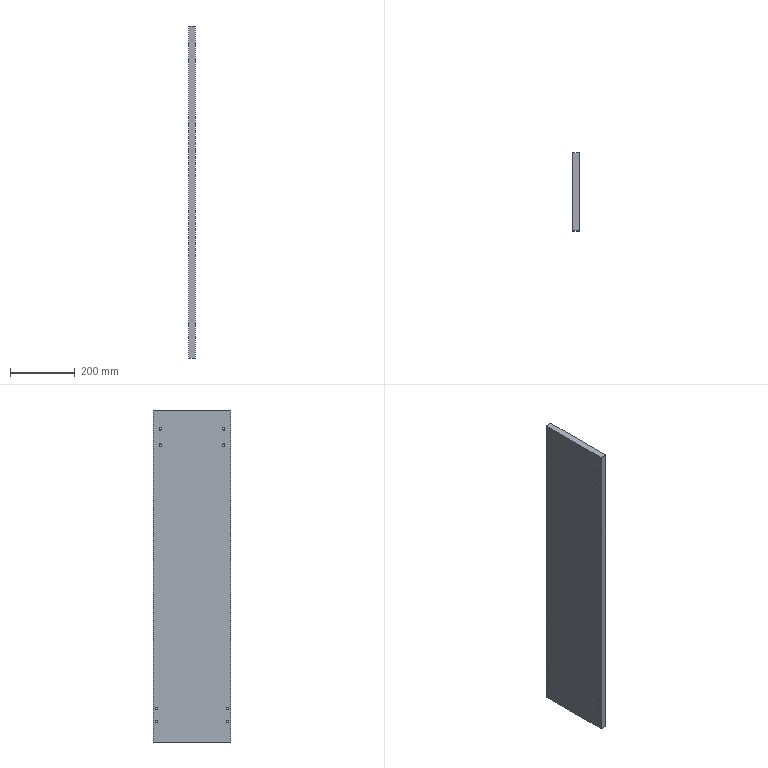Part | NX | features SIMPLE HOLE 8, SYMBOLIC_THREAD 8, LINKED_CURVE 4, DATUM_CSYS 3, SKETCH 2, EXTRUDE 1, HOLE PACKAGE 1, LINKED_FACE 1 | 1 solid | 30 faces | box 20 x 240 x 1027 mm | volume 4923724 mm3 | cone 16 | cylinder 8 | plane 6 | commonest cylinder face diameters 6.8 x8
STEP:
#1=CARTESIAN_POINT('',(85.,-120.,527.));
#2=VERTEX_POINT('',#1);
#3=CARTESIAN_POINT('',(85.,-120.,-500.));
#4=VERTEX_POINT('',#3);
#5=CARTESIAN_POINT('',(85.,-120.,527.));
#6=DIRECTION('',(0.,0.,-1.));
#7=VECTOR('',#6,1000.);
#8=LINE('',#5,#7);
#9=EDGE_CURVE('',#2,#4,#8,.T.);
#10=ORIENTED_EDGE('',*,*,#9,.T.);
#11=CARTESIAN_POINT('',(105.,-120.,-500.));
#12=VERTEX_POINT('',#11);
#13=CARTESIAN_POINT('',(105.,-120.,-500.));
#14=DIRECTION('',(-1.,0.,0.));
#15=VECTOR('',#14,1000.);
#16=LINE('',#13,#15);
#17=EDGE_CURVE('',#12,#4,#16,.T.);
#18=ORIENTED_EDGE('',*,*,#17,.F.);
#19=CARTESIAN_POINT('',(105.,-120.,527.));
#20=VERTEX_POINT('',#19);
#21=CARTESIAN_POINT('',(105.,-120.,527.));
#22=DIRECTION('',(0.,0.,-1.));
#23=VECTOR('',#22,1000.);
#24=LINE('',#21,#23);
#25=EDGE_CURVE('',#20,#12,#24,.T.);
#26=ORIENTED_EDGE('',*,*,#25,.F.);
#27=CARTESIAN_POINT('',(105.,-120.,527.));
#28=DIRECTION('',(-1.,0.,0.));
#29=VECTOR('',#28,1000.);
#30=LINE('',#27,#29);
#31=EDGE_CURVE('',#20,#2,#30,.T.);
#32=ORIENTED_EDGE('',*,*,#31,.T.);
#33=EDGE_LOOP('',(#10,#18,#26,#32));
#34=FACE_BOUND('',#33,.T.);
#35=CARTESIAN_POINT('',(105.,-120.,527.));
#36=DIRECTION('',(0.,1.,0.));
#37=DIRECTION('',(0.,0.,1.));
#38=AXIS2_PLACEMENT_3D('',#35,#36,#37);
#39=PLANE('',#38);
#40=ADVANCED_FACE('',(#34),#39,.F.);
#41=CARTESIAN_POINT('',(85.,120.,-500.));
#42=VERTEX_POINT('',#41);
#43=CARTESIAN_POINT('',(85.,-120.,-500.));
#44=DIRECTION('',(0.,1.,0.));
#45=VECTOR('',#44,1000.);
#46=LINE('',#43,#45);
#47=EDGE_CURVE('',#4,#42,#46,.T.);
#48=ORIENTED_EDGE('',*,*,#47,.T.);
#49=CARTESIAN_POINT('',(105.,120.,-500.));
#50=VERTEX_POINT('',#49);
#51=CARTESIAN_POINT('',(105.,120.,-500.));
#52=DIRECTION('',(-1.,0.,0.));
#53=VECTOR('',#52,1000.);
#54=LINE('',#51,#53);
#55=EDGE_CURVE('',#50,#42,#54,.T.);
#56=ORIENTED_EDGE('',*,*,#55,.F.);
#57=CARTESIAN_POINT('',(105.,-120.,-500.));
#58=DIRECTION('',(0.,1.,0.));
#59=VECTOR('',#58,1000.);
#60=LINE('',#57,#59);
#61=EDGE_CURVE('',#12,#50,#60,.T.);
#62=ORIENTED_EDGE('',*,*,#61,.F.);
#63=ORIENTED_EDGE('',*,*,#17,.T.);
#64=EDGE_LOOP('',(#48,#56,#62,#63));
#65=FACE_BOUND('',#64,.T.);
#66=CARTESIAN_POINT('',(105.,-120.,-500.));
#67=DIRECTION('',(0.,0.,1.));
#68=DIRECTION('',(1.,0.,0.));
#69=AXIS2_PLACEMENT_3D('',#66,#67,#68);
#70=PLANE('',#69);
#71=ADVANCED_FACE('',(#65),#70,.F.);
#72=CARTESIAN_POINT('',(85.,120.,527.));
#73=VERTEX_POINT('',#72);
#74=CARTESIAN_POINT('',(85.,120.,-500.));
#75=DIRECTION('',(0.,0.,1.));
#76=VECTOR('',#75,1000.);
#77=LINE('',#74,#76);
#78=EDGE_CURVE('',#42,#73,#77,.T.);
#79=ORIENTED_EDGE('',*,*,#78,.T.);
#80=CARTESIAN_POINT('',(105.,120.,527.));
#81=VERTEX_POINT('',#80);
#82=CARTESIAN_POINT('',(105.,120.,527.));
#83=DIRECTION('',(-1.,0.,0.));
#84=VECTOR('',#83,1000.);
#85=LINE('',#82,#84);
#86=EDGE_CURVE('',#81,#73,#85,.T.);
#87=ORIENTED_EDGE('',*,*,#86,.F.);
#88=CARTESIAN_POINT('',(105.,120.,-500.));
#89=DIRECTION('',(0.,0.,1.));
#90=VECTOR('',#89,1000.);
#91=LINE('',#88,#90);
#92=EDGE_CURVE('',#50,#81,#91,.T.);
#93=ORIENTED_EDGE('',*,*,#92,.F.);
#94=ORIENTED_EDGE('',*,*,#55,.T.);
#95=EDGE_LOOP('',(#79,#87,#93,#94));
#96=FACE_BOUND('',#95,.T.);
#97=CARTESIAN_POINT('',(105.,120.,-500.));
#98=DIRECTION('',(0.,-1.,0.));
#99=DIRECTION('',(0.,0.,-1.));
#100=AXIS2_PLACEMENT_3D('',#97,#98,#99);
#101=PLANE('',#100);
#102=ADVANCED_FACE('',(#96),#101,.F.);
#103=CARTESIAN_POINT('',(85.,120.,527.));
#104=DIRECTION('',(0.,-1.,0.));
#105=VECTOR('',#104,1000.);
#106=LINE('',#103,#105);
#107=EDGE_CURVE('',#73,#2,#106,.T.);
#108=ORIENTED_EDGE('',*,*,#107,.T.);
#109=ORIENTED_EDGE('',*,*,#31,.F.);
#110=CARTESIAN_POINT('',(105.,120.,527.));
#111=DIRECTION('',(0.,-1.,0.));
#112=VECTOR('',#111,1000.);
#113=LINE('',#110,#112);
#114=EDGE_CURVE('',#81,#20,#113,.T.);
#115=ORIENTED_EDGE('',*,*,#114,.F.);
#116=ORIENTED_EDGE('',*,*,#86,.T.);
#117=EDGE_LOOP('',(#108,#109,#115,#116));
#118=FACE_BOUND('',#117,.T.);
#119=CARTESIAN_POINT('',(105.,120.,527.));
#120=DIRECTION('',(0.,0.,-1.));
#121=DIRECTION('',(-1.,0.,0.));
#122=AXIS2_PLACEMENT_3D('',#119,#120,#121);
#123=PLANE('',#122);
#124=ADVANCED_FACE('',(#118),#123,.F.);
#125=CARTESIAN_POINT('',(105.,110.,-400.5));
#126=VERTEX_POINT('',#125);
#127=CARTESIAN_POINT('',(105.,110.,-396.5));
#128=DIRECTION('',(1.,0.,0.));
#129=DIRECTION('',(0.,0.,-1.));
#130=AXIS2_PLACEMENT_3D('',#127,#128,#129);
#131=CIRCLE('',#130,4.);
#132=EDGE_CURVE('',#126,#126,#131,.F.);
#133=ORIENTED_EDGE('',*,*,#132,.T.);
#134=EDGE_LOOP('',(#133));
#135=FACE_BOUND('',#134,.T.);
#136=CARTESIAN_POINT('',(105.,110.,-440.5));
#137=VERTEX_POINT('',#136);
#138=CARTESIAN_POINT('',(105.,110.,-436.5));
#139=DIRECTION('',(1.,0.,0.));
#140=DIRECTION('',(0.,0.,-1.));
#141=AXIS2_PLACEMENT_3D('',#138,#139,#140);
#142=CIRCLE('',#141,4.);
#143=EDGE_CURVE('',#137,#137,#142,.F.);
#144=ORIENTED_EDGE('',*,*,#143,.T.);
#145=EDGE_LOOP('',(#144));
#146=FACE_BOUND('',#145,.T.);
#147=CARTESIAN_POINT('',(105.,98.,464.5));
#148=VERTEX_POINT('',#147);
#149=CARTESIAN_POINT('',(105.,98.,468.5));
#150=DIRECTION('',(1.,0.,0.));
#151=DIRECTION('',(0.,0.,-1.));
#152=AXIS2_PLACEMENT_3D('',#149,#150,#151);
#153=CIRCLE('',#152,4.);
#154=EDGE_CURVE('',#148,#148,#153,.F.);
#155=ORIENTED_EDGE('',*,*,#154,.T.);
#156=EDGE_LOOP('',(#155));
#157=FACE_BOUND('',#156,.T.);
#158=CARTESIAN_POINT('',(105.,98.,414.5));
#159=VERTEX_POINT('',#158);
#160=CARTESIAN_POINT('',(105.,98.,418.5));
#161=DIRECTION('',(1.,0.,0.));
#162=DIRECTION('',(0.,0.,-1.));
#163=AXIS2_PLACEMENT_3D('',#160,#161,#162);
#164=CIRCLE('',#163,4.);
#165=EDGE_CURVE('',#159,#159,#164,.F.);
#166=ORIENTED_EDGE('',*,*,#165,.T.);
#167=EDGE_LOOP('',(#166));
#168=FACE_BOUND('',#167,.T.);
#169=CARTESIAN_POINT('',(105.,-98.,464.5));
#170=VERTEX_POINT('',#169);
#171=CARTESIAN_POINT('',(105.,-98.,468.5));
#172=DIRECTION('',(1.,0.,0.));
#173=DIRECTION('',(0.,0.,-1.));
#174=AXIS2_PLACEMENT_3D('',#171,#172,#173);
#175=CIRCLE('',#174,4.);
#176=EDGE_CURVE('',#170,#170,#175,.F.);
#177=ORIENTED_EDGE('',*,*,#176,.T.);
#178=EDGE_LOOP('',(#177));
#179=FACE_BOUND('',#178,.T.);
#180=CARTESIAN_POINT('',(105.,-98.,414.5));
#181=VERTEX_POINT('',#180);
#182=CARTESIAN_POINT('',(105.,-98.,418.5));
#183=DIRECTION('',(1.,0.,0.));
#184=DIRECTION('',(0.,0.,-1.));
#185=AXIS2_PLACEMENT_3D('',#182,#183,#184);
#186=CIRCLE('',#185,4.);
#187=EDGE_CURVE('',#181,#181,#186,.F.);
#188=ORIENTED_EDGE('',*,*,#187,.T.);
#189=EDGE_LOOP('',(#188));
#190=FACE_BOUND('',#189,.T.);
#191=CARTESIAN_POINT('',(105.,-110.,-400.5));
#192=VERTEX_POINT('',#191);
#193=CARTESIAN_POINT('',(105.,-110.,-396.5));
#194=DIRECTION('',(1.,0.,0.));
#195=DIRECTION('',(0.,0.,-1.));
#196=AXIS2_PLACEMENT_3D('',#193,#194,#195);
#197=CIRCLE('',#196,4.);
#198=EDGE_CURVE('',#192,#192,#197,.F.);
#199=ORIENTED_EDGE('',*,*,#198,.T.);
#200=EDGE_LOOP('',(#199));
#201=FACE_BOUND('',#200,.T.);
#202=CARTESIAN_POINT('',(105.,-110.,-440.5));
#203=VERTEX_POINT('',#202);
#204=CARTESIAN_POINT('',(105.,-110.,-436.5));
#205=DIRECTION('',(1.,0.,0.));
#206=DIRECTION('',(0.,0.,-1.));
#207=AXIS2_PLACEMENT_3D('',#204,#205,#206);
#208=CIRCLE('',#207,4.);
#209=EDGE_CURVE('',#203,#203,#208,.F.);
#210=ORIENTED_EDGE('',*,*,#209,.T.);
#211=EDGE_LOOP('',(#210));
#212=FACE_BOUND('',#211,.T.);
#213=ORIENTED_EDGE('',*,*,#25,.T.);
#214=ORIENTED_EDGE('',*,*,#61,.T.);
#215=ORIENTED_EDGE('',*,*,#92,.T.);
#216=ORIENTED_EDGE('',*,*,#114,.T.);
#217=EDGE_LOOP('',(#213,#214,#215,#216));
#218=FACE_BOUND('',#217,.T.);
#219=CARTESIAN_POINT('',(105.,0.,0.));
#220=DIRECTION('',(1.,0.,0.));
#221=DIRECTION('',(0.,0.,-1.));
#222=AXIS2_PLACEMENT_3D('',#219,#220,#221);
#223=PLANE('',#222);
#224=ADVANCED_FACE('',(#135,#146,#157,#168,#179,#190,#201,#212,#218),#223,.T.);
#225=CARTESIAN_POINT('',(85.,110.,-400.5));
#226=VERTEX_POINT('',#225);
#227=CARTESIAN_POINT('',(85.,110.,-396.5));
#228=DIRECTION('',(1.,0.,0.));
#229=DIRECTION('',(0.,0.,-1.));
#230=AXIS2_PLACEMENT_3D('',#227,#228,#229);
#231=CIRCLE('',#230,4.);
#232=EDGE_CURVE('',#226,#226,#231,.T.);
#233=ORIENTED_EDGE('',*,*,#232,.T.);
#234=EDGE_LOOP('',(#233));
#235=FACE_BOUND('',#234,.T.);
#236=CARTESIAN_POINT('',(85.,110.,-440.5));
#237=VERTEX_POINT('',#236);
#238=CARTESIAN_POINT('',(85.,110.,-436.5));
#239=DIRECTION('',(1.,0.,0.));
#240=DIRECTION('',(0.,0.,-1.));
#241=AXIS2_PLACEMENT_3D('',#238,#239,#240);
#242=CIRCLE('',#241,4.);
#243=EDGE_CURVE('',#237,#237,#242,.T.);
#244=ORIENTED_EDGE('',*,*,#243,.T.);
#245=EDGE_LOOP('',(#244));
#246=FACE_BOUND('',#245,.T.);
#247=CARTESIAN_POINT('',(85.,98.,464.5));
#248=VERTEX_POINT('',#247);
#249=CARTESIAN_POINT('',(85.,98.,468.5));
#250=DIRECTION('',(1.,0.,0.));
#251=DIRECTION('',(0.,0.,-1.));
#252=AXIS2_PLACEMENT_3D('',#249,#250,#251);
#253=CIRCLE('',#252,4.);
#254=EDGE_CURVE('',#248,#248,#253,.T.);
#255=ORIENTED_EDGE('',*,*,#254,.T.);
#256=EDGE_LOOP('',(#255));
#257=FACE_BOUND('',#256,.T.);
#258=CARTESIAN_POINT('',(85.,98.,414.5));
#259=VERTEX_POINT('',#258);
#260=CARTESIAN_POINT('',(85.,98.,418.5));
#261=DIRECTION('',(1.,0.,0.));
#262=DIRECTION('',(0.,0.,-1.));
#263=AXIS2_PLACEMENT_3D('',#260,#261,#262);
#264=CIRCLE('',#263,4.);
#265=EDGE_CURVE('',#259,#259,#264,.T.);
#266=ORIENTED_EDGE('',*,*,#265,.T.);
#267=EDGE_LOOP('',(#266));
#268=FACE_BOUND('',#267,.T.);
#269=CARTESIAN_POINT('',(85.,-98.,464.5));
#270=VERTEX_POINT('',#269);
#271=CARTESIAN_POINT('',(85.,-98.,468.5));
#272=DIRECTION('',(1.,0.,0.));
#273=DIRECTION('',(0.,0.,-1.));
#274=AXIS2_PLACEMENT_3D('',#271,#272,#273);
#275=CIRCLE('',#274,4.);
#276=EDGE_CURVE('',#270,#270,#275,.T.);
#277=ORIENTED_EDGE('',*,*,#276,.T.);
#278=EDGE_LOOP('',(#277));
#279=FACE_BOUND('',#278,.T.);
#280=CARTESIAN_POINT('',(85.,-98.,414.5));
#281=VERTEX_POINT('',#280);
#282=CARTESIAN_POINT('',(85.,-98.,418.5));
#283=DIRECTION('',(1.,0.,0.));
#284=DIRECTION('',(0.,0.,-1.));
#285=AXIS2_PLACEMENT_3D('',#282,#283,#284);
#286=CIRCLE('',#285,4.);
#287=EDGE_CURVE('',#281,#281,#286,.T.);
#288=ORIENTED_EDGE('',*,*,#287,.T.);
#289=EDGE_LOOP('',(#288));
#290=FACE_BOUND('',#289,.T.);
#291=CARTESIAN_POINT('',(85.,-110.,-400.5));
#292=VERTEX_POINT('',#291);
#293=CARTESIAN_POINT('',(85.,-110.,-396.5));
#294=DIRECTION('',(1.,0.,0.));
#295=DIRECTION('',(0.,0.,-1.));
#296=AXIS2_PLACEMENT_3D('',#293,#294,#295);
#297=CIRCLE('',#296,4.);
#298=EDGE_CURVE('',#292,#292,#297,.T.);
#299=ORIENTED_EDGE('',*,*,#298,.T.);
#300=EDGE_LOOP('',(#299));
#301=FACE_BOUND('',#300,.T.);
#302=CARTESIAN_POINT('',(85.,-110.,-440.5));
#303=VERTEX_POINT('',#302);
#304=CARTESIAN_POINT('',(85.,-110.,-436.5));
#305=DIRECTION('',(1.,0.,0.));
#306=DIRECTION('',(0.,0.,-1.));
#307=AXIS2_PLACEMENT_3D('',#304,#305,#306);
#308=CIRCLE('',#307,4.);
#309=EDGE_CURVE('',#303,#303,#308,.T.);
#310=ORIENTED_EDGE('',*,*,#309,.T.);
#311=EDGE_LOOP('',(#310));
#312=FACE_BOUND('',#311,.T.);
#313=ORIENTED_EDGE('',*,*,#9,.F.);
#314=ORIENTED_EDGE('',*,*,#107,.F.);
#315=ORIENTED_EDGE('',*,*,#78,.F.);
#316=ORIENTED_EDGE('',*,*,#47,.F.);
#317=EDGE_LOOP('',(#313,#314,#315,#316));
#318=FACE_BOUND('',#317,.T.);
#319=CARTESIAN_POINT('',(85.,0.,0.));
#320=DIRECTION('',(1.,0.,0.));
#321=DIRECTION('',(0.,0.,-1.));
#322=AXIS2_PLACEMENT_3D('',#319,#320,#321);
#323=PLANE('',#322);
#324=ADVANCED_FACE('',(#235,#246,#257,#268,#279,#290,#301,#312,#318),#323,.F.);
#325=CARTESIAN_POINT('',(104.4,-110.,-439.9));
#326=VERTEX_POINT('',#325);
#327=CARTESIAN_POINT('',(104.4,-110.,-436.5));
#328=DIRECTION('',(1.,0.,0.));
#329=DIRECTION('',(0.,0.,-1.));
#330=AXIS2_PLACEMENT_3D('',#327,#328,#329);
#331=CIRCLE('',#330,3.4);
#332=EDGE_CURVE('',#326,#326,#331,.T.);
#333=ORIENTED_EDGE('',*,*,#332,.T.);
#334=EDGE_LOOP('',(#333));
#335=FACE_BOUND('',#334,.T.);
#336=CARTESIAN_POINT('',(85.6,-110.,-439.9));
#337=VERTEX_POINT('',#336);
#338=CARTESIAN_POINT('',(85.6,-110.,-436.5));
#339=DIRECTION('',(1.,0.,0.));
#340=DIRECTION('',(0.,0.,-1.));
#341=AXIS2_PLACEMENT_3D('',#338,#339,#340);
#342=CIRCLE('',#341,3.4);
#343=EDGE_CURVE('',#337,#337,#342,.F.);
#344=ORIENTED_EDGE('',*,*,#343,.T.);
#345=EDGE_LOOP('',(#344));
#346=FACE_BOUND('',#345,.T.);
#347=CARTESIAN_POINT('',(85.,-110.,-436.5));
#348=DIRECTION('',(1.,0.,0.));
#349=DIRECTION('',(0.,0.,-1.));
#350=AXIS2_PLACEMENT_3D('',#347,#348,#349);
#351=CYLINDRICAL_SURFACE('',#350,3.4);
#352=ADVANCED_FACE('',(#335,#346),#351,.F.);
#353=ORIENTED_EDGE('',*,*,#343,.F.);
#354=EDGE_LOOP('',(#353));
#355=FACE_BOUND('',#354,.T.);
#356=ORIENTED_EDGE('',*,*,#309,.F.);
#357=EDGE_LOOP('',(#356));
#358=FACE_BOUND('',#357,.T.);
#359=CARTESIAN_POINT('',(85.,-110.,-436.5));
#360=DIRECTION('',(-1.,0.,0.));
#361=DIRECTION('',(0.,0.,1.));
#362=AXIS2_PLACEMENT_3D('',#359,#360,#361);
#363=CONICAL_SURFACE('',#362,4.,0.7854);
#364=ADVANCED_FACE('',(#355,#358),#363,.F.);
#365=ORIENTED_EDGE('',*,*,#209,.F.);
#366=EDGE_LOOP('',(#365));
#367=FACE_BOUND('',#366,.T.);
#368=ORIENTED_EDGE('',*,*,#332,.F.);
#369=EDGE_LOOP('',(#368));
#370=FACE_BOUND('',#369,.T.);
#371=CARTESIAN_POINT('',(104.4,-110.,-436.5));
#372=DIRECTION('',(1.,0.,0.));
#373=DIRECTION('',(0.,0.,-1.));
#374=AXIS2_PLACEMENT_3D('',#371,#372,#373);
#375=CONICAL_SURFACE('',#374,3.4,0.7854);
#376=ADVANCED_FACE('',(#367,#370),#375,.F.);
#377=CARTESIAN_POINT('',(104.4,-110.,-399.9));
#378=VERTEX_POINT('',#377);
#379=CARTESIAN_POINT('',(104.4,-110.,-396.5));
#380=DIRECTION('',(1.,0.,0.));
#381=DIRECTION('',(0.,0.,-1.));
#382=AXIS2_PLACEMENT_3D('',#379,#380,#381);
#383=CIRCLE('',#382,3.4);
#384=EDGE_CURVE('',#378,#378,#383,.T.);
#385=ORIENTED_EDGE('',*,*,#384,.T.);
#386=EDGE_LOOP('',(#385));
#387=FACE_BOUND('',#386,.T.);
#388=CARTESIAN_POINT('',(85.6,-110.,-399.9));
#389=VERTEX_POINT('',#388);
#390=CARTESIAN_POINT('',(85.6,-110.,-396.5));
#391=DIRECTION('',(1.,0.,0.));
#392=DIRECTION('',(0.,0.,-1.));
#393=AXIS2_PLACEMENT_3D('',#390,#391,#392);
#394=CIRCLE('',#393,3.4);
#395=EDGE_CURVE('',#389,#389,#394,.F.);
#396=ORIENTED_EDGE('',*,*,#395,.T.);
#397=EDGE_LOOP('',(#396));
#398=FACE_BOUND('',#397,.T.);
#399=CARTESIAN_POINT('',(85.,-110.,-396.5));
#400=DIRECTION('',(1.,0.,0.));
#401=DIRECTION('',(0.,0.,-1.));
#402=AXIS2_PLACEMENT_3D('',#399,#400,#401);
#403=CYLINDRICAL_SURFACE('',#402,3.4);
#404=ADVANCED_FACE('',(#387,#398),#403,.F.);
#405=ORIENTED_EDGE('',*,*,#395,.F.);
#406=EDGE_LOOP('',(#405));
#407=FACE_BOUND('',#406,.T.);
#408=ORIENTED_EDGE('',*,*,#298,.F.);
#409=EDGE_LOOP('',(#408));
#410=FACE_BOUND('',#409,.T.);
#411=CARTESIAN_POINT('',(85.,-110.,-396.5));
#412=DIRECTION('',(-1.,0.,0.));
#413=DIRECTION('',(0.,0.,1.));
#414=AXIS2_PLACEMENT_3D('',#411,#412,#413);
#415=CONICAL_SURFACE('',#414,4.,0.7854);
#416=ADVANCED_FACE('',(#407,#410),#415,.F.);
#417=ORIENTED_EDGE('',*,*,#198,.F.);
#418=EDGE_LOOP('',(#417));
#419=FACE_BOUND('',#418,.T.);
#420=ORIENTED_EDGE('',*,*,#384,.F.);
#421=EDGE_LOOP('',(#420));
#422=FACE_BOUND('',#421,.T.);
#423=CARTESIAN_POINT('',(104.4,-110.,-396.5));
#424=DIRECTION('',(1.,0.,0.));
#425=DIRECTION('',(0.,0.,-1.));
#426=AXIS2_PLACEMENT_3D('',#423,#424,#425);
#427=CONICAL_SURFACE('',#426,3.4,0.7854);
#428=ADVANCED_FACE('',(#419,#422),#427,.F.);
#429=CARTESIAN_POINT('',(104.4,-98.,415.1));
#430=VERTEX_POINT('',#429);
#431=CARTESIAN_POINT('',(104.4,-98.,418.5));
#432=DIRECTION('',(1.,0.,0.));
#433=DIRECTION('',(0.,0.,-1.));
#434=AXIS2_PLACEMENT_3D('',#431,#432,#433);
#435=CIRCLE('',#434,3.4);
#436=EDGE_CURVE('',#430,#430,#435,.T.);
#437=ORIENTED_EDGE('',*,*,#436,.T.);
#438=EDGE_LOOP('',(#437));
#439=FACE_BOUND('',#438,.T.);
#440=CARTESIAN_POINT('',(85.6,-98.,415.1));
#441=VERTEX_POINT('',#440);
#442=CARTESIAN_POINT('',(85.6,-98.,418.5));
#443=DIRECTION('',(1.,0.,0.));
#444=DIRECTION('',(0.,0.,-1.));
#445=AXIS2_PLACEMENT_3D('',#442,#443,#444);
#446=CIRCLE('',#445,3.4);
#447=EDGE_CURVE('',#441,#441,#446,.F.);
#448=ORIENTED_EDGE('',*,*,#447,.T.);
#449=EDGE_LOOP('',(#448));
#450=FACE_BOUND('',#449,.T.);
#451=CARTESIAN_POINT('',(85.,-98.,418.5));
#452=DIRECTION('',(1.,0.,0.));
#453=DIRECTION('',(0.,0.,-1.));
#454=AXIS2_PLACEMENT_3D('',#451,#452,#453);
#455=CYLINDRICAL_SURFACE('',#454,3.4);
#456=ADVANCED_FACE('',(#439,#450),#455,.F.);
#457=ORIENTED_EDGE('',*,*,#447,.F.);
#458=EDGE_LOOP('',(#457));
#459=FACE_BOUND('',#458,.T.);
#460=ORIENTED_EDGE('',*,*,#287,.F.);
#461=EDGE_LOOP('',(#460));
#462=FACE_BOUND('',#461,.T.);
#463=CARTESIAN_POINT('',(85.,-98.,418.5));
#464=DIRECTION('',(-1.,0.,0.));
#465=DIRECTION('',(0.,0.,1.));
#466=AXIS2_PLACEMENT_3D('',#463,#464,#465);
#467=CONICAL_SURFACE('',#466,4.,0.7854);
#468=ADVANCED_FACE('',(#459,#462),#467,.F.);
#469=ORIENTED_EDGE('',*,*,#187,.F.);
#470=EDGE_LOOP('',(#469));
#471=FACE_BOUND('',#470,.T.);
#472=ORIENTED_EDGE('',*,*,#436,.F.);
#473=EDGE_LOOP('',(#472));
#474=FACE_BOUND('',#473,.T.);
#475=CARTESIAN_POINT('',(104.4,-98.,418.5));
#476=DIRECTION('',(1.,0.,0.));
#477=DIRECTION('',(0.,0.,-1.));
#478=AXIS2_PLACEMENT_3D('',#475,#476,#477);
#479=CONICAL_SURFACE('',#478,3.4,0.7854);
#480=ADVANCED_FACE('',(#471,#474),#479,.F.);
#481=CARTESIAN_POINT('',(104.4,-98.,465.1));
#482=VERTEX_POINT('',#481);
#483=CARTESIAN_POINT('',(104.4,-98.,468.5));
#484=DIRECTION('',(1.,0.,0.));
#485=DIRECTION('',(0.,0.,-1.));
#486=AXIS2_PLACEMENT_3D('',#483,#484,#485);
#487=CIRCLE('',#486,3.4);
#488=EDGE_CURVE('',#482,#482,#487,.T.);
#489=ORIENTED_EDGE('',*,*,#488,.T.);
#490=EDGE_LOOP('',(#489));
#491=FACE_BOUND('',#490,.T.);
#492=CARTESIAN_POINT('',(85.6,-98.,465.1));
#493=VERTEX_POINT('',#492);
#494=CARTESIAN_POINT('',(85.6,-98.,468.5));
#495=DIRECTION('',(1.,0.,0.));
#496=DIRECTION('',(0.,0.,-1.));
#497=AXIS2_PLACEMENT_3D('',#494,#495,#496);
#498=CIRCLE('',#497,3.4);
#499=EDGE_CURVE('',#493,#493,#498,.F.);
#500=ORIENTED_EDGE('',*,*,#499,.T.);
#501=EDGE_LOOP('',(#500));
#502=FACE_BOUND('',#501,.T.);
#503=CARTESIAN_POINT('',(85.,-98.,468.5));
#504=DIRECTION('',(1.,0.,0.));
#505=DIRECTION('',(0.,0.,-1.));
#506=AXIS2_PLACEMENT_3D('',#503,#504,#505);
#507=CYLINDRICAL_SURFACE('',#506,3.4);
#508=ADVANCED_FACE('',(#491,#502),#507,.F.);
#509=ORIENTED_EDGE('',*,*,#499,.F.);
#510=EDGE_LOOP('',(#509));
#511=FACE_BOUND('',#510,.T.);
#512=ORIENTED_EDGE('',*,*,#276,.F.);
#513=EDGE_LOOP('',(#512));
#514=FACE_BOUND('',#513,.T.);
#515=CARTESIAN_POINT('',(85.,-98.,468.5));
#516=DIRECTION('',(-1.,0.,0.));
#517=DIRECTION('',(0.,0.,1.));
#518=AXIS2_PLACEMENT_3D('',#515,#516,#517);
#519=CONICAL_SURFACE('',#518,4.,0.7854);
#520=ADVANCED_FACE('',(#511,#514),#519,.F.);
#521=ORIENTED_EDGE('',*,*,#176,.F.);
#522=EDGE_LOOP('',(#521));
#523=FACE_BOUND('',#522,.T.);
#524=ORIENTED_EDGE('',*,*,#488,.F.);
#525=EDGE_LOOP('',(#524));
#526=FACE_BOUND('',#525,.T.);
#527=CARTESIAN_POINT('',(104.4,-98.,468.5));
#528=DIRECTION('',(1.,0.,0.));
#529=DIRECTION('',(0.,0.,-1.));
#530=AXIS2_PLACEMENT_3D('',#527,#528,#529);
#531=CONICAL_SURFACE('',#530,3.4,0.7854);
#532=ADVANCED_FACE('',(#523,#526),#531,.F.);
#533=CARTESIAN_POINT('',(104.4,98.,415.1));
#534=VERTEX_POINT('',#533);
#535=CARTESIAN_POINT('',(104.4,98.,418.5));
#536=DIRECTION('',(1.,0.,0.));
#537=DIRECTION('',(0.,0.,-1.));
#538=AXIS2_PLACEMENT_3D('',#535,#536,#537);
#539=CIRCLE('',#538,3.4);
#540=EDGE_CURVE('',#534,#534,#539,.T.);
#541=ORIENTED_EDGE('',*,*,#540,.T.);
#542=EDGE_LOOP('',(#541));
#543=FACE_BOUND('',#542,.T.);
#544=CARTESIAN_POINT('',(85.6,98.,415.1));
#545=VERTEX_POINT('',#544);
#546=CARTESIAN_POINT('',(85.6,98.,418.5));
#547=DIRECTION('',(1.,0.,0.));
#548=DIRECTION('',(0.,0.,-1.));
#549=AXIS2_PLACEMENT_3D('',#546,#547,#548);
#550=CIRCLE('',#549,3.4);
#551=EDGE_CURVE('',#545,#545,#550,.F.);
#552=ORIENTED_EDGE('',*,*,#551,.T.);
#553=EDGE_LOOP('',(#552));
#554=FACE_BOUND('',#553,.T.);
#555=CARTESIAN_POINT('',(85.,98.,418.5));
#556=DIRECTION('',(1.,0.,0.));
#557=DIRECTION('',(0.,0.,-1.));
#558=AXIS2_PLACEMENT_3D('',#555,#556,#557);
#559=CYLINDRICAL_SURFACE('',#558,3.4);
#560=ADVANCED_FACE('',(#543,#554),#559,.F.);
#561=ORIENTED_EDGE('',*,*,#551,.F.);
#562=EDGE_LOOP('',(#561));
#563=FACE_BOUND('',#562,.T.);
#564=ORIENTED_EDGE('',*,*,#265,.F.);
#565=EDGE_LOOP('',(#564));
#566=FACE_BOUND('',#565,.T.);
#567=CARTESIAN_POINT('',(85.,98.,418.5));
#568=DIRECTION('',(-1.,0.,0.));
#569=DIRECTION('',(0.,0.,1.));
#570=AXIS2_PLACEMENT_3D('',#567,#568,#569);
#571=CONICAL_SURFACE('',#570,4.,0.7854);
#572=ADVANCED_FACE('',(#563,#566),#571,.F.);
#573=ORIENTED_EDGE('',*,*,#165,.F.);
#574=EDGE_LOOP('',(#573));
#575=FACE_BOUND('',#574,.T.);
#576=ORIENTED_EDGE('',*,*,#540,.F.);
#577=EDGE_LOOP('',(#576));
#578=FACE_BOUND('',#577,.T.);
#579=CARTESIAN_POINT('',(104.4,98.,418.5));
#580=DIRECTION('',(1.,0.,0.));
#581=DIRECTION('',(0.,0.,-1.));
#582=AXIS2_PLACEMENT_3D('',#579,#580,#581);
#583=CONICAL_SURFACE('',#582,3.4,0.7854);
#584=ADVANCED_FACE('',(#575,#578),#583,.F.);
#585=CARTESIAN_POINT('',(104.4,98.,465.1));
#586=VERTEX_POINT('',#585);
#587=CARTESIAN_POINT('',(104.4,98.,468.5));
#588=DIRECTION('',(1.,0.,0.));
#589=DIRECTION('',(0.,0.,-1.));
#590=AXIS2_PLACEMENT_3D('',#587,#588,#589);
#591=CIRCLE('',#590,3.4);
#592=EDGE_CURVE('',#586,#586,#591,.T.);
#593=ORIENTED_EDGE('',*,*,#592,.T.);
#594=EDGE_LOOP('',(#593));
#595=FACE_BOUND('',#594,.T.);
#596=CARTESIAN_POINT('',(85.6,98.,465.1));
#597=VERTEX_POINT('',#596);
#598=CARTESIAN_POINT('',(85.6,98.,468.5));
#599=DIRECTION('',(1.,0.,0.));
#600=DIRECTION('',(0.,0.,-1.));
#601=AXIS2_PLACEMENT_3D('',#598,#599,#600);
#602=CIRCLE('',#601,3.4);
#603=EDGE_CURVE('',#597,#597,#602,.F.);
#604=ORIENTED_EDGE('',*,*,#603,.T.);
#605=EDGE_LOOP('',(#604));
#606=FACE_BOUND('',#605,.T.);
#607=CARTESIAN_POINT('',(85.,98.,468.5));
#608=DIRECTION('',(1.,0.,0.));
#609=DIRECTION('',(0.,0.,-1.));
#610=AXIS2_PLACEMENT_3D('',#607,#608,#609);
#611=CYLINDRICAL_SURFACE('',#610,3.4);
#612=ADVANCED_FACE('',(#595,#606),#611,.F.);
#613=ORIENTED_EDGE('',*,*,#603,.F.);
#614=EDGE_LOOP('',(#613));
#615=FACE_BOUND('',#614,.T.);
#616=ORIENTED_EDGE('',*,*,#254,.F.);
#617=EDGE_LOOP('',(#616));
#618=FACE_BOUND('',#617,.T.);
#619=CARTESIAN_POINT('',(85.,98.,468.5));
#620=DIRECTION('',(-1.,0.,0.));
#621=DIRECTION('',(0.,0.,1.));
#622=AXIS2_PLACEMENT_3D('',#619,#620,#621);
#623=CONICAL_SURFACE('',#622,4.,0.7854);
#624=ADVANCED_FACE('',(#615,#618),#623,.F.);
#625=ORIENTED_EDGE('',*,*,#154,.F.);
#626=EDGE_LOOP('',(#625));
#627=FACE_BOUND('',#626,.T.);
#628=ORIENTED_EDGE('',*,*,#592,.F.);
#629=EDGE_LOOP('',(#628));
#630=FACE_BOUND('',#629,.T.);
#631=CARTESIAN_POINT('',(104.4,98.,468.5));
#632=DIRECTION('',(1.,0.,0.));
#633=DIRECTION('',(0.,0.,-1.));
#634=AXIS2_PLACEMENT_3D('',#631,#632,#633);
#635=CONICAL_SURFACE('',#634,3.4,0.7854);
#636=ADVANCED_FACE('',(#627,#630),#635,.F.);
#637=CARTESIAN_POINT('',(104.4,110.,-439.9));
#638=VERTEX_POINT('',#637);
#639=CARTESIAN_POINT('',(104.4,110.,-436.5));
#640=DIRECTION('',(1.,0.,0.));
#641=DIRECTION('',(0.,0.,-1.));
#642=AXIS2_PLACEMENT_3D('',#639,#640,#641);
#643=CIRCLE('',#642,3.4);
#644=EDGE_CURVE('',#638,#638,#643,.T.);
#645=ORIENTED_EDGE('',*,*,#644,.T.);
#646=EDGE_LOOP('',(#645));
#647=FACE_BOUND('',#646,.T.);
#648=CARTESIAN_POINT('',(85.6,110.,-439.9));
#649=VERTEX_POINT('',#648);
#650=CARTESIAN_POINT('',(85.6,110.,-436.5));
#651=DIRECTION('',(1.,0.,0.));
#652=DIRECTION('',(0.,0.,-1.));
#653=AXIS2_PLACEMENT_3D('',#650,#651,#652);
#654=CIRCLE('',#653,3.4);
#655=EDGE_CURVE('',#649,#649,#654,.F.);
#656=ORIENTED_EDGE('',*,*,#655,.T.);
#657=EDGE_LOOP('',(#656));
#658=FACE_BOUND('',#657,.T.);
#659=CARTESIAN_POINT('',(85.,110.,-436.5));
#660=DIRECTION('',(1.,0.,0.));
#661=DIRECTION('',(0.,0.,-1.));
#662=AXIS2_PLACEMENT_3D('',#659,#660,#661);
#663=CYLINDRICAL_SURFACE('',#662,3.4);
#664=ADVANCED_FACE('',(#647,#658),#663,.F.);
#665=ORIENTED_EDGE('',*,*,#655,.F.);
#666=EDGE_LOOP('',(#665));
#667=FACE_BOUND('',#666,.T.);
#668=ORIENTED_EDGE('',*,*,#243,.F.);
#669=EDGE_LOOP('',(#668));
#670=FACE_BOUND('',#669,.T.);
#671=CARTESIAN_POINT('',(85.,110.,-436.5));
#672=DIRECTION('',(-1.,0.,0.));
#673=DIRECTION('',(0.,0.,1.));
#674=AXIS2_PLACEMENT_3D('',#671,#672,#673);
#675=CONICAL_SURFACE('',#674,4.,0.7854);
#676=ADVANCED_FACE('',(#667,#670),#675,.F.);
#677=ORIENTED_EDGE('',*,*,#143,.F.);
#678=EDGE_LOOP('',(#677));
#679=FACE_BOUND('',#678,.T.);
#680=ORIENTED_EDGE('',*,*,#644,.F.);
#681=EDGE_LOOP('',(#680));
#682=FACE_BOUND('',#681,.T.);
#683=CARTESIAN_POINT('',(104.4,110.,-436.5));
#684=DIRECTION('',(1.,0.,0.));
#685=DIRECTION('',(0.,0.,-1.));
#686=AXIS2_PLACEMENT_3D('',#683,#684,#685);
#687=CONICAL_SURFACE('',#686,3.4,0.7854);
#688=ADVANCED_FACE('',(#679,#682),#687,.F.);
#689=CARTESIAN_POINT('',(104.4,110.,-399.9));
#690=VERTEX_POINT('',#689);
#691=CARTESIAN_POINT('',(104.4,110.,-396.5));
#692=DIRECTION('',(1.,0.,0.));
#693=DIRECTION('',(0.,0.,-1.));
#694=AXIS2_PLACEMENT_3D('',#691,#692,#693);
#695=CIRCLE('',#694,3.4);
#696=EDGE_CURVE('',#690,#690,#695,.T.);
#697=ORIENTED_EDGE('',*,*,#696,.T.);
#698=EDGE_LOOP('',(#697));
#699=FACE_BOUND('',#698,.T.);
#700=CARTESIAN_POINT('',(85.6,110.,-399.9));
#701=VERTEX_POINT('',#700);
#702=CARTESIAN_POINT('',(85.6,110.,-396.5));
#703=DIRECTION('',(1.,0.,0.));
#704=DIRECTION('',(0.,0.,-1.));
#705=AXIS2_PLACEMENT_3D('',#702,#703,#704);
#706=CIRCLE('',#705,3.4);
#707=EDGE_CURVE('',#701,#701,#706,.F.);
#708=ORIENTED_EDGE('',*,*,#707,.T.);
#709=EDGE_LOOP('',(#708));
#710=FACE_BOUND('',#709,.T.);
#711=CARTESIAN_POINT('',(85.,110.,-396.5));
#712=DIRECTION('',(1.,0.,0.));
#713=DIRECTION('',(0.,0.,-1.));
#714=AXIS2_PLACEMENT_3D('',#711,#712,#713);
#715=CYLINDRICAL_SURFACE('',#714,3.4);
#716=ADVANCED_FACE('',(#699,#710),#715,.F.);
#717=ORIENTED_EDGE('',*,*,#707,.F.);
#718=EDGE_LOOP('',(#717));
#719=FACE_BOUND('',#718,.T.);
#720=ORIENTED_EDGE('',*,*,#232,.F.);
#721=EDGE_LOOP('',(#720));
#722=FACE_BOUND('',#721,.T.);
#723=CARTESIAN_POINT('',(85.,110.,-396.5));
#724=DIRECTION('',(-1.,0.,0.));
#725=DIRECTION('',(0.,0.,1.));
#726=AXIS2_PLACEMENT_3D('',#723,#724,#725);
#727=CONICAL_SURFACE('',#726,4.,0.7854);
#728=ADVANCED_FACE('',(#719,#722),#727,.F.);
#729=ORIENTED_EDGE('',*,*,#132,.F.);
#730=EDGE_LOOP('',(#729));
#731=FACE_BOUND('',#730,.T.);
#732=ORIENTED_EDGE('',*,*,#696,.F.);
#733=EDGE_LOOP('',(#732));
#734=FACE_BOUND('',#733,.T.);
#735=CARTESIAN_POINT('',(104.4,110.,-396.5));
#736=DIRECTION('',(1.,0.,0.));
#737=DIRECTION('',(0.,0.,-1.));
#738=AXIS2_PLACEMENT_3D('',#735,#736,#737);
#739=CONICAL_SURFACE('',#738,3.4,0.7854);
#740=ADVANCED_FACE('',(#731,#734),#739,.F.);
#741=CLOSED_SHELL('',(#40,#71,#102,#124,#224,#324,#352,#364,#376,#404,#416,#428,#456,#468,#480,#508,#520,#532,#560,#572,#584,#612,#624,#636,#664,#676,#688,#716,#728,#740));
#742=MANIFOLD_SOLID_BREP('',#741);
#743=(LENGTH_UNIT()NAMED_UNIT(*)SI_UNIT(.MILLI.,.METRE.));
#744=UNCERTAINTY_MEASURE_WITH_UNIT(LENGTH_MEASURE(0.00001),#743,'','');
#745=(NAMED_UNIT(*)PLANE_ANGLE_UNIT()SI_UNIT($,.RADIAN.));
#746=(NAMED_UNIT(*)SI_UNIT($,.STERADIAN.)SOLID_ANGLE_UNIT());
#747=(GEOMETRIC_REPRESENTATION_CONTEXT(3)GLOBAL_UNCERTAINTY_ASSIGNED_CONTEXT((#744))GLOBAL_UNIT_ASSIGNED_CONTEXT((#743,#745,#746))REPRESENTATION_CONTEXT('',''));
#748=ADVANCED_BREP_SHAPE_REPRESENTATION('',(#742),#747);